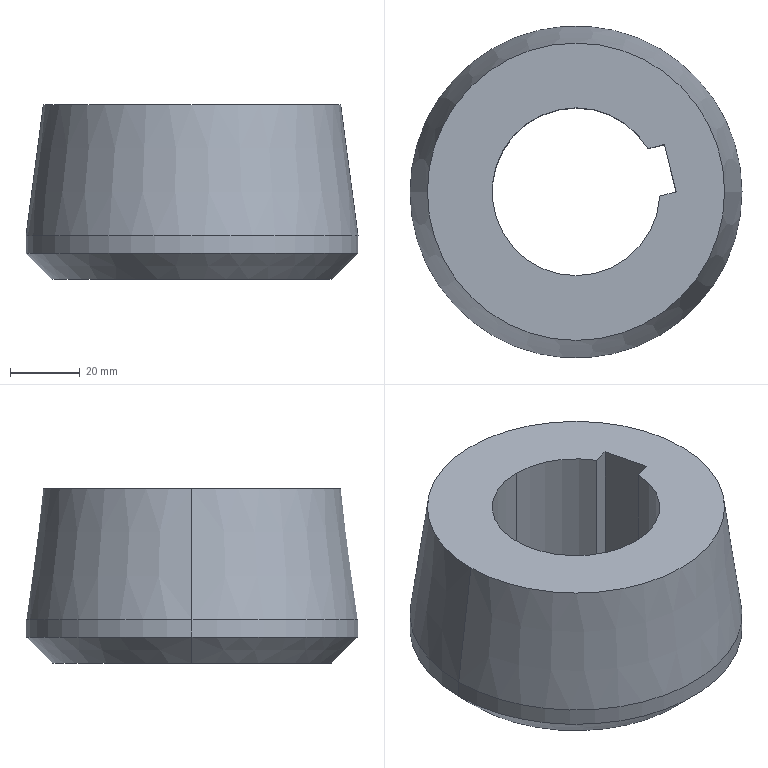Part | SolidWorks | features ICE 1, RevCut 1, Revolution 1 | 1 solid | 14 faces | box 95 x 95 x 50 mm | volume 226212 mm3 | cylinder 5 | plane 5 | cone 4 | commonest cylinder face diameters 48 x3 95 x2
STEP:
#1=CARTESIAN_POINT('',(521.231,210.744,-774.998));
#2=VERTEX_POINT('',#1);
#3=CARTESIAN_POINT('',(521.231,258.744,-774.998));
#4=VERTEX_POINT('',#3);
#5=CARTESIAN_POINT('',(521.231,234.744,-774.998));
#6=DIRECTION('',(0.,0.,-1.));
#7=DIRECTION('',(0.,1.,0.));
#8=AXIS2_PLACEMENT_3D('',#5,#6,#7);
#9=CIRCLE('',#8,24.);
#10=EDGE_CURVE('',#2,#4,#9,.T.);
#11=ORIENTED_EDGE('',*,*,#10,.F.);
#12=CARTESIAN_POINT('',(521.231,210.744,-824.998));
#13=VERTEX_POINT('',#12);
#14=CARTESIAN_POINT('',(521.231,210.744,-774.998));
#15=DIRECTION('',(0.,0.,-1.));
#16=VECTOR('',#15,1000.);
#17=LINE('',#14,#16);
#18=EDGE_CURVE('',#2,#13,#17,.T.);
#19=ORIENTED_EDGE('',*,*,#18,.T.);
#20=CARTESIAN_POINT('',(521.231,258.744,-824.998));
#21=VERTEX_POINT('',#20);
#22=CARTESIAN_POINT('',(521.231,234.744,-824.998));
#23=DIRECTION('',(0.,0.,-1.));
#24=DIRECTION('',(0.,1.,0.));
#25=AXIS2_PLACEMENT_3D('',#22,#23,#24);
#26=CIRCLE('',#25,24.);
#27=EDGE_CURVE('',#13,#21,#26,.T.);
#28=ORIENTED_EDGE('',*,*,#27,.T.);
#29=CARTESIAN_POINT('',(521.231,258.744,-774.998));
#30=DIRECTION('',(0.,0.,-1.));
#31=VECTOR('',#30,1000.);
#32=LINE('',#29,#31);
#33=EDGE_CURVE('',#4,#21,#32,.T.);
#34=ORIENTED_EDGE('',*,*,#33,.F.);
#35=EDGE_LOOP('',(#11,#19,#28,#34));
#36=FACE_OUTER_BOUND('',#35,.T.);
#37=CARTESIAN_POINT('',(521.231,234.744,-774.998));
#38=DIRECTION('',(0.,0.,-1.));
#39=DIRECTION('',(0.,1.,0.));
#40=AXIS2_PLACEMENT_3D('',#37,#38,#39);
#41=CYLINDRICAL_SURFACE('',#40,24.);
#42=ADVANCED_FACE('',(#36),#41,.F.);
#43=CARTESIAN_POINT('',(541.805,247.101,-774.998));
#44=VERTEX_POINT('',#43);
#45=CARTESIAN_POINT('',(521.231,234.744,-774.998));
#46=DIRECTION('',(0.,0.,-1.));
#47=DIRECTION('',(0.,1.,0.));
#48=AXIS2_PLACEMENT_3D('',#45,#46,#47);
#49=CIRCLE('',#48,24.);
#50=EDGE_CURVE('',#4,#44,#49,.T.);
#51=ORIENTED_EDGE('',*,*,#50,.F.);
#52=ORIENTED_EDGE('',*,*,#33,.T.);
#53=CARTESIAN_POINT('',(541.805,247.101,-824.998));
#54=VERTEX_POINT('',#53);
#55=CARTESIAN_POINT('',(521.231,234.744,-824.998));
#56=DIRECTION('',(0.,0.,-1.));
#57=DIRECTION('',(0.,1.,0.));
#58=AXIS2_PLACEMENT_3D('',#55,#56,#57);
#59=CIRCLE('',#58,24.);
#60=EDGE_CURVE('',#21,#54,#59,.T.);
#61=ORIENTED_EDGE('',*,*,#60,.T.);
#62=CARTESIAN_POINT('',(541.805,247.101,-824.998));
#63=DIRECTION('',(0.,0.,1.));
#64=VECTOR('',#63,1000.);
#65=LINE('',#62,#64);
#66=EDGE_CURVE('',#54,#44,#65,.T.);
#67=ORIENTED_EDGE('',*,*,#66,.T.);
#68=EDGE_LOOP('',(#51,#52,#61,#67));
#69=FACE_OUTER_BOUND('',#68,.T.);
#70=CARTESIAN_POINT('',(521.231,234.744,-774.998));
#71=DIRECTION('',(0.,0.,-1.));
#72=DIRECTION('',(0.,1.,0.));
#73=AXIS2_PLACEMENT_3D('',#70,#71,#72);
#74=CYLINDRICAL_SURFACE('',#73,24.);
#75=ADVANCED_FACE('',(#69),#74,.F.);
#76=CARTESIAN_POINT('',(563.756,234.744,-774.998));
#77=VERTEX_POINT('',#76);
#78=CARTESIAN_POINT('',(478.706,234.744,-774.998));
#79=VERTEX_POINT('',#78);
#80=CARTESIAN_POINT('',(521.231,234.744,-774.998));
#81=DIRECTION('',(0.,0.,1.));
#82=DIRECTION('',(1.,0.,0.));
#83=AXIS2_PLACEMENT_3D('',#80,#81,#82);
#84=CIRCLE('',#83,42.525);
#85=EDGE_CURVE('',#77,#79,#84,.T.);
#86=ORIENTED_EDGE('',*,*,#85,.F.);
#87=CARTESIAN_POINT('',(568.731,234.744,-812.498));
#88=VERTEX_POINT('',#87);
#89=CARTESIAN_POINT('',(563.756,234.744,-774.998));
#90=DIRECTION('',(0.1315,0.,-0.9913));
#91=VECTOR('',#90,1000.);
#92=LINE('',#89,#91);
#93=EDGE_CURVE('',#77,#88,#92,.T.);
#94=ORIENTED_EDGE('',*,*,#93,.T.);
#95=CARTESIAN_POINT('',(473.731,234.744,-812.498));
#96=VERTEX_POINT('',#95);
#97=CARTESIAN_POINT('',(521.231,234.744,-812.498));
#98=DIRECTION('',(0.,0.,1.));
#99=DIRECTION('',(1.,0.,0.));
#100=AXIS2_PLACEMENT_3D('',#97,#98,#99);
#101=CIRCLE('',#100,47.5);
#102=EDGE_CURVE('',#88,#96,#101,.T.);
#103=ORIENTED_EDGE('',*,*,#102,.T.);
#104=CARTESIAN_POINT('',(478.706,234.744,-774.998));
#105=DIRECTION('',(-0.1315,0.,-0.9913));
#106=VECTOR('',#105,1000.);
#107=LINE('',#104,#106);
#108=EDGE_CURVE('',#79,#96,#107,.T.);
#109=ORIENTED_EDGE('',*,*,#108,.F.);
#110=EDGE_LOOP('',(#86,#94,#103,#109));
#111=FACE_OUTER_BOUND('',#110,.T.);
#112=CARTESIAN_POINT('',(521.231,234.744,-774.998));
#113=DIRECTION('',(0.,0.,-1.));
#114=DIRECTION('',(-1.,0.,0.));
#115=AXIS2_PLACEMENT_3D('',#112,#113,#114);
#116=CONICAL_SURFACE('',#115,42.525,0.1319);
#117=ADVANCED_FACE('',(#111),#116,.T.);
#118=CARTESIAN_POINT('',(568.731,234.744,-817.498));
#119=VERTEX_POINT('',#118);
#120=CARTESIAN_POINT('',(473.731,234.744,-817.498));
#121=VERTEX_POINT('',#120);
#122=CARTESIAN_POINT('',(521.231,234.744,-817.498));
#123=DIRECTION('',(0.,0.,1.));
#124=DIRECTION('',(1.,0.,0.));
#125=AXIS2_PLACEMENT_3D('',#122,#123,#124);
#126=CIRCLE('',#125,47.5);
#127=EDGE_CURVE('',#119,#121,#126,.T.);
#128=ORIENTED_EDGE('',*,*,#127,.T.);
#129=CARTESIAN_POINT('',(473.731,234.744,-824.998));
#130=DIRECTION('',(0.,0.,1.));
#131=VECTOR('',#130,1000.);
#132=LINE('',#129,#131);
#133=EDGE_CURVE('',#121,#96,#132,.T.);
#134=ORIENTED_EDGE('',*,*,#133,.T.);
#135=ORIENTED_EDGE('',*,*,#102,.F.);
#136=CARTESIAN_POINT('',(568.731,234.744,-824.998));
#137=DIRECTION('',(0.,0.,1.));
#138=VECTOR('',#137,1000.);
#139=LINE('',#136,#138);
#140=EDGE_CURVE('',#119,#88,#139,.T.);
#141=ORIENTED_EDGE('',*,*,#140,.F.);
#142=EDGE_LOOP('',(#128,#134,#135,#141));
#143=FACE_OUTER_BOUND('',#142,.T.);
#144=CARTESIAN_POINT('',(521.231,234.744,-824.998));
#145=DIRECTION('',(0.,0.,1.));
#146=DIRECTION('',(1.,0.,0.));
#147=AXIS2_PLACEMENT_3D('',#144,#145,#146);
#148=CYLINDRICAL_SURFACE('',#147,47.5);
#149=ADVANCED_FACE('',(#143),#148,.T.);
#150=CARTESIAN_POINT('',(561.231,234.744,-824.998));
#151=VERTEX_POINT('',#150);
#152=CARTESIAN_POINT('',(481.231,234.744,-824.998));
#153=VERTEX_POINT('',#152);
#154=CARTESIAN_POINT('',(521.231,234.744,-824.998));
#155=DIRECTION('',(0.,0.,1.));
#156=DIRECTION('',(1.,0.,0.));
#157=AXIS2_PLACEMENT_3D('',#154,#155,#156);
#158=CIRCLE('',#157,40.);
#159=EDGE_CURVE('',#151,#153,#158,.T.);
#160=ORIENTED_EDGE('',*,*,#159,.T.);
#161=CARTESIAN_POINT('',(473.731,234.744,-817.498));
#162=DIRECTION('',(-0.7071,0.,0.7071));
#163=VECTOR('',#162,1000.);
#164=LINE('',#161,#163);
#165=EDGE_CURVE('',#153,#121,#164,.T.);
#166=ORIENTED_EDGE('',*,*,#165,.T.);
#167=ORIENTED_EDGE('',*,*,#127,.F.);
#168=CARTESIAN_POINT('',(568.731,234.744,-817.498));
#169=DIRECTION('',(0.7071,0.,0.7071));
#170=VECTOR('',#169,1000.);
#171=LINE('',#168,#170);
#172=EDGE_CURVE('',#151,#119,#171,.T.);
#173=ORIENTED_EDGE('',*,*,#172,.F.);
#174=EDGE_LOOP('',(#160,#166,#167,#173));
#175=FACE_OUTER_BOUND('',#174,.T.);
#176=CARTESIAN_POINT('',(521.231,234.744,-817.498));
#177=DIRECTION('',(0.,0.,1.));
#178=DIRECTION('',(1.,0.,0.));
#179=AXIS2_PLACEMENT_3D('',#176,#177,#178);
#180=CONICAL_SURFACE('',#179,47.5,0.7854);
#181=ADVANCED_FACE('',(#175),#180,.T.);
#182=ORIENTED_EDGE('',*,*,#165,.F.);
#183=CARTESIAN_POINT('',(521.231,234.744,-824.998));
#184=DIRECTION('',(0.,0.,1.));
#185=DIRECTION('',(1.,0.,0.));
#186=AXIS2_PLACEMENT_3D('',#183,#184,#185);
#187=CIRCLE('',#186,40.);
#188=EDGE_CURVE('',#153,#151,#187,.T.);
#189=ORIENTED_EDGE('',*,*,#188,.T.);
#190=ORIENTED_EDGE('',*,*,#172,.T.);
#191=CARTESIAN_POINT('',(521.231,234.744,-817.498));
#192=DIRECTION('',(0.,0.,1.));
#193=DIRECTION('',(1.,0.,0.));
#194=AXIS2_PLACEMENT_3D('',#191,#192,#193);
#195=CIRCLE('',#194,47.5);
#196=EDGE_CURVE('',#121,#119,#195,.T.);
#197=ORIENTED_EDGE('',*,*,#196,.F.);
#198=EDGE_LOOP('',(#182,#189,#190,#197));
#199=FACE_OUTER_BOUND('',#198,.T.);
#200=CARTESIAN_POINT('',(521.231,234.744,-817.498));
#201=DIRECTION('',(0.,0.,1.));
#202=DIRECTION('',(1.,0.,0.));
#203=AXIS2_PLACEMENT_3D('',#200,#201,#202);
#204=CONICAL_SURFACE('',#203,47.5,0.7854);
#205=ADVANCED_FACE('',(#199),#204,.T.);
#206=ORIENTED_EDGE('',*,*,#133,.F.);
#207=ORIENTED_EDGE('',*,*,#196,.T.);
#208=ORIENTED_EDGE('',*,*,#140,.T.);
#209=CARTESIAN_POINT('',(521.231,234.744,-812.498));
#210=DIRECTION('',(0.,0.,1.));
#211=DIRECTION('',(1.,0.,0.));
#212=AXIS2_PLACEMENT_3D('',#209,#210,#211);
#213=CIRCLE('',#212,47.5);
#214=EDGE_CURVE('',#96,#88,#213,.T.);
#215=ORIENTED_EDGE('',*,*,#214,.F.);
#216=EDGE_LOOP('',(#206,#207,#208,#215));
#217=FACE_OUTER_BOUND('',#216,.T.);
#218=CARTESIAN_POINT('',(521.231,234.744,-824.998));
#219=DIRECTION('',(0.,0.,1.));
#220=DIRECTION('',(1.,0.,0.));
#221=AXIS2_PLACEMENT_3D('',#218,#219,#220);
#222=CYLINDRICAL_SURFACE('',#221,47.5);
#223=ADVANCED_FACE('',(#217),#222,.T.);
#224=ORIENTED_EDGE('',*,*,#93,.F.);
#225=CARTESIAN_POINT('',(521.231,234.744,-774.998));
#226=DIRECTION('',(0.,0.,1.));
#227=DIRECTION('',(1.,0.,0.));
#228=AXIS2_PLACEMENT_3D('',#225,#226,#227);
#229=CIRCLE('',#228,42.525);
#230=EDGE_CURVE('',#79,#77,#229,.T.);
#231=ORIENTED_EDGE('',*,*,#230,.F.);
#232=ORIENTED_EDGE('',*,*,#108,.T.);
#233=ORIENTED_EDGE('',*,*,#214,.T.);
#234=EDGE_LOOP('',(#224,#231,#232,#233));
#235=FACE_OUTER_BOUND('',#234,.T.);
#236=CARTESIAN_POINT('',(521.231,234.744,-774.998));
#237=DIRECTION('',(0.,0.,-1.));
#238=DIRECTION('',(-1.,0.,0.));
#239=AXIS2_PLACEMENT_3D('',#236,#237,#238);
#240=CONICAL_SURFACE('',#239,42.525,0.1319);
#241=ADVANCED_FACE('',(#235),#240,.T.);
#242=CARTESIAN_POINT('',(545.199,233.519,-774.998));
#243=VERTEX_POINT('',#242);
#244=CARTESIAN_POINT('',(521.231,234.744,-774.998));
#245=DIRECTION('',(0.,0.,-1.));
#246=DIRECTION('',(0.,1.,0.));
#247=AXIS2_PLACEMENT_3D('',#244,#245,#246);
#248=CIRCLE('',#247,24.);
#249=EDGE_CURVE('',#243,#2,#248,.T.);
#250=ORIENTED_EDGE('',*,*,#249,.T.);
#251=ORIENTED_EDGE('',*,*,#10,.T.);
#252=ORIENTED_EDGE('',*,*,#50,.T.);
#253=CARTESIAN_POINT('',(546.504,248.275,-774.998));
#254=VERTEX_POINT('',#253);
#255=CARTESIAN_POINT('',(546.504,248.275,-774.998));
#256=DIRECTION('',(-0.9702,-0.2424,0.));
#257=VECTOR('',#256,1000.);
#258=LINE('',#255,#257);
#259=EDGE_CURVE('',#254,#44,#258,.T.);
#260=ORIENTED_EDGE('',*,*,#259,.F.);
#261=CARTESIAN_POINT('',(549.898,234.693,-774.998));
#262=VERTEX_POINT('',#261);
#263=CARTESIAN_POINT('',(549.898,234.693,-774.998));
#264=DIRECTION('',(-0.2424,0.9702,0.));
#265=VECTOR('',#264,1000.);
#266=LINE('',#263,#265);
#267=EDGE_CURVE('',#262,#254,#266,.T.);
#268=ORIENTED_EDGE('',*,*,#267,.F.);
#269=CARTESIAN_POINT('',(545.199,233.519,-774.998));
#270=DIRECTION('',(0.9702,0.2424,0.));
#271=VECTOR('',#270,1000.);
#272=LINE('',#269,#271);
#273=EDGE_CURVE('',#243,#262,#272,.T.);
#274=ORIENTED_EDGE('',*,*,#273,.F.);
#275=EDGE_LOOP('',(#250,#251,#252,#260,#268,#274));
#276=FACE_BOUND('',#275,.T.);
#277=ORIENTED_EDGE('',*,*,#230,.T.);
#278=ORIENTED_EDGE('',*,*,#85,.T.);
#279=EDGE_LOOP('',(#277,#278));
#280=FACE_OUTER_BOUND('',#279,.T.);
#281=CARTESIAN_POINT('',(521.231,234.744,-774.998));
#282=DIRECTION('',(0.,0.,1.));
#283=DIRECTION('',(1.,0.,0.));
#284=AXIS2_PLACEMENT_3D('',#281,#282,#283);
#285=PLANE('',#284);
#286=ADVANCED_FACE('',(#276,#280),#285,.T.);
#287=CARTESIAN_POINT('',(545.199,233.519,-824.998));
#288=VERTEX_POINT('',#287);
#289=CARTESIAN_POINT('',(521.231,234.744,-824.998));
#290=DIRECTION('',(0.,0.,-1.));
#291=DIRECTION('',(0.,1.,0.));
#292=AXIS2_PLACEMENT_3D('',#289,#290,#291);
#293=CIRCLE('',#292,24.);
#294=EDGE_CURVE('',#288,#13,#293,.T.);
#295=ORIENTED_EDGE('',*,*,#294,.F.);
#296=CARTESIAN_POINT('',(549.898,234.693,-824.998));
#297=VERTEX_POINT('',#296);
#298=CARTESIAN_POINT('',(545.199,233.519,-824.998));
#299=DIRECTION('',(0.9702,0.2424,0.));
#300=VECTOR('',#299,1000.);
#301=LINE('',#298,#300);
#302=EDGE_CURVE('',#288,#297,#301,.T.);
#303=ORIENTED_EDGE('',*,*,#302,.T.);
#304=CARTESIAN_POINT('',(546.504,248.275,-824.998));
#305=VERTEX_POINT('',#304);
#306=CARTESIAN_POINT('',(549.898,234.693,-824.998));
#307=DIRECTION('',(-0.2424,0.9702,0.));
#308=VECTOR('',#307,1000.);
#309=LINE('',#306,#308);
#310=EDGE_CURVE('',#297,#305,#309,.T.);
#311=ORIENTED_EDGE('',*,*,#310,.T.);
#312=CARTESIAN_POINT('',(546.504,248.275,-824.998));
#313=DIRECTION('',(-0.9702,-0.2424,0.));
#314=VECTOR('',#313,1000.);
#315=LINE('',#312,#314);
#316=EDGE_CURVE('',#305,#54,#315,.T.);
#317=ORIENTED_EDGE('',*,*,#316,.T.);
#318=ORIENTED_EDGE('',*,*,#60,.F.);
#319=ORIENTED_EDGE('',*,*,#27,.F.);
#320=EDGE_LOOP('',(#295,#303,#311,#317,#318,#319));
#321=FACE_BOUND('',#320,.T.);
#322=ORIENTED_EDGE('',*,*,#159,.F.);
#323=ORIENTED_EDGE('',*,*,#188,.F.);
#324=EDGE_LOOP('',(#322,#323));
#325=FACE_OUTER_BOUND('',#324,.T.);
#326=CARTESIAN_POINT('',(561.231,234.744,-824.998));
#327=DIRECTION('',(0.,0.,-1.));
#328=DIRECTION('',(-1.,0.,0.));
#329=AXIS2_PLACEMENT_3D('',#326,#327,#328);
#330=PLANE('',#329);
#331=ADVANCED_FACE('',(#321,#325),#330,.T.);
#332=ORIENTED_EDGE('',*,*,#273,.T.);
#333=CARTESIAN_POINT('',(549.898,234.693,-824.998));
#334=DIRECTION('',(0.,0.,1.));
#335=VECTOR('',#334,1000.);
#336=LINE('',#333,#335);
#337=EDGE_CURVE('',#297,#262,#336,.T.);
#338=ORIENTED_EDGE('',*,*,#337,.F.);
#339=ORIENTED_EDGE('',*,*,#302,.F.);
#340=CARTESIAN_POINT('',(545.199,233.519,-824.998));
#341=DIRECTION('',(0.,0.,1.));
#342=VECTOR('',#341,1000.);
#343=LINE('',#340,#342);
#344=EDGE_CURVE('',#288,#243,#343,.T.);
#345=ORIENTED_EDGE('',*,*,#344,.T.);
#346=EDGE_LOOP('',(#332,#338,#339,#345));
#347=FACE_OUTER_BOUND('',#346,.T.);
#348=CARTESIAN_POINT('',(545.199,233.519,-824.998));
#349=DIRECTION('',(0.2424,-0.9702,0.));
#350=DIRECTION('',(0.9702,0.2424,0.));
#351=AXIS2_PLACEMENT_3D('',#348,#349,#350);
#352=PLANE('',#351);
#353=ADVANCED_FACE('',(#347),#352,.F.);
#354=ORIENTED_EDGE('',*,*,#259,.T.);
#355=ORIENTED_EDGE('',*,*,#66,.F.);
#356=ORIENTED_EDGE('',*,*,#316,.F.);
#357=CARTESIAN_POINT('',(546.504,248.275,-824.998));
#358=DIRECTION('',(0.,0.,1.));
#359=VECTOR('',#358,1000.);
#360=LINE('',#357,#359);
#361=EDGE_CURVE('',#305,#254,#360,.T.);
#362=ORIENTED_EDGE('',*,*,#361,.T.);
#363=EDGE_LOOP('',(#354,#355,#356,#362));
#364=FACE_OUTER_BOUND('',#363,.T.);
#365=CARTESIAN_POINT('',(546.504,248.275,-824.998));
#366=DIRECTION('',(-0.2424,0.9702,0.));
#367=DIRECTION('',(-0.9702,-0.2424,0.));
#368=AXIS2_PLACEMENT_3D('',#365,#366,#367);
#369=PLANE('',#368);
#370=ADVANCED_FACE('',(#364),#369,.F.);
#371=ORIENTED_EDGE('',*,*,#267,.T.);
#372=ORIENTED_EDGE('',*,*,#361,.F.);
#373=ORIENTED_EDGE('',*,*,#310,.F.);
#374=ORIENTED_EDGE('',*,*,#337,.T.);
#375=EDGE_LOOP('',(#371,#372,#373,#374));
#376=FACE_OUTER_BOUND('',#375,.T.);
#377=CARTESIAN_POINT('',(549.898,234.693,-824.998));
#378=DIRECTION('',(0.9702,0.2424,0.));
#379=DIRECTION('',(-0.2424,0.9702,0.));
#380=AXIS2_PLACEMENT_3D('',#377,#378,#379);
#381=PLANE('',#380);
#382=ADVANCED_FACE('',(#376),#381,.F.);
#383=ORIENTED_EDGE('',*,*,#18,.F.);
#384=ORIENTED_EDGE('',*,*,#249,.F.);
#385=ORIENTED_EDGE('',*,*,#344,.F.);
#386=ORIENTED_EDGE('',*,*,#294,.T.);
#387=EDGE_LOOP('',(#383,#384,#385,#386));
#388=FACE_OUTER_BOUND('',#387,.T.);
#389=CARTESIAN_POINT('',(521.231,234.744,-774.998));
#390=DIRECTION('',(0.,0.,-1.));
#391=DIRECTION('',(0.,1.,0.));
#392=AXIS2_PLACEMENT_3D('',#389,#390,#391);
#393=CYLINDRICAL_SURFACE('',#392,24.);
#394=ADVANCED_FACE('',(#388),#393,.F.);
#395=CLOSED_SHELL('',(#42,#75,#117,#149,#181,#205,#223,#241,#286,#331,#353,#370,#382,#394));
#396=MANIFOLD_SOLID_BREP('',#395);
#397=CARTESIAN_POINT('',(0.,0.,0.));
#398=DIRECTION('',(0.,0.,1.));
#399=DIRECTION('',(1.,0.,0.));
#400=AXIS2_PLACEMENT_3D('',#397,#398,#399);
#401=(LENGTH_UNIT()NAMED_UNIT(*)SI_UNIT(.MILLI.,.METRE.));
#402=UNCERTAINTY_MEASURE_WITH_UNIT(LENGTH_MEASURE(0.00001),#401,'','');
#403=(NAMED_UNIT(*)PLANE_ANGLE_UNIT()SI_UNIT($,.RADIAN.));
#404=(NAMED_UNIT(*)SI_UNIT($,.STERADIAN.)SOLID_ANGLE_UNIT());
#405=(GEOMETRIC_REPRESENTATION_CONTEXT(3)GLOBAL_UNCERTAINTY_ASSIGNED_CONTEXT((#402))GLOBAL_UNIT_ASSIGNED_CONTEXT((#401,#403,#404))REPRESENTATION_CONTEXT('',''));
#406=ADVANCED_BREP_SHAPE_REPRESENTATION('',(#396,#400),#405);